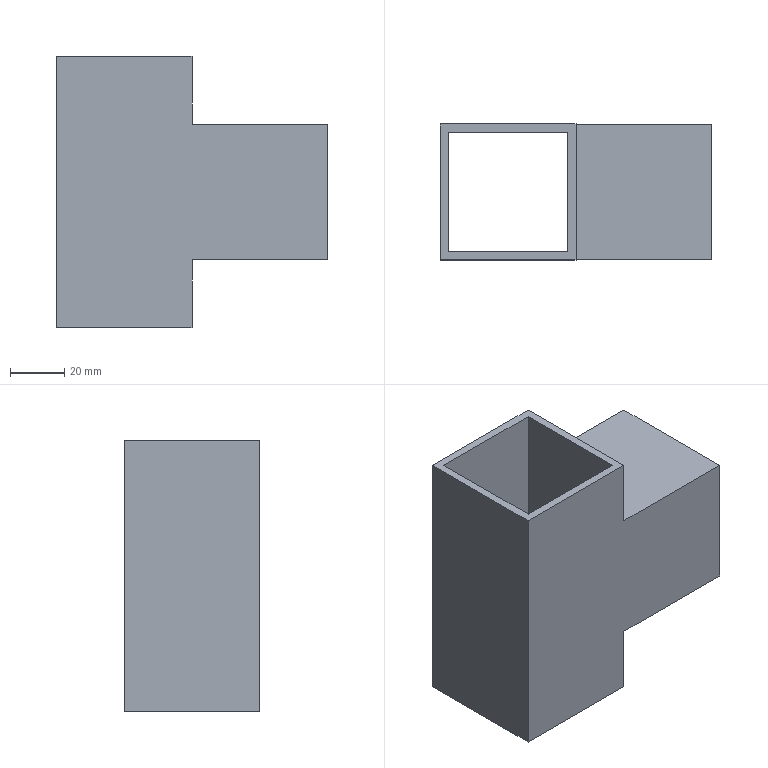Part | SolidWorks | features ICE 3, Extrusion 1 | 1 solid | 19 faces | box 100 x 50 x 100 mm | volume 84600 mm3 | plane 19
STEP:
#1=CARTESIAN_POINT('',(50.,0.,100.));
#2=VERTEX_POINT('',#1);
#3=CARTESIAN_POINT('',(50.,0.,75.));
#4=VERTEX_POINT('',#3);
#5=CARTESIAN_POINT('',(50.,0.,200.));
#6=DIRECTION('',(0.,0.,-1.));
#7=VECTOR('',#6,1000.);
#8=LINE('',#5,#7);
#9=EDGE_CURVE('',#2,#4,#8,.T.);
#10=ORIENTED_EDGE('',*,*,#9,.T.);
#11=CARTESIAN_POINT('',(50.,50.,75.));
#12=VERTEX_POINT('',#11);
#13=CARTESIAN_POINT('',(50.,50.,75.));
#14=DIRECTION('',(0.,1.,0.));
#15=VECTOR('',#14,1000.);
#16=LINE('',#13,#15);
#17=EDGE_CURVE('',#4,#12,#16,.T.);
#18=ORIENTED_EDGE('',*,*,#17,.T.);
#19=CARTESIAN_POINT('',(50.,50.,100.));
#20=VERTEX_POINT('',#19);
#21=CARTESIAN_POINT('',(50.,50.,200.));
#22=DIRECTION('',(0.,0.,-1.));
#23=VECTOR('',#22,1000.);
#24=LINE('',#21,#23);
#25=EDGE_CURVE('',#20,#12,#24,.T.);
#26=ORIENTED_EDGE('',*,*,#25,.F.);
#27=CARTESIAN_POINT('',(50.,50.,100.));
#28=DIRECTION('',(0.,1.,0.));
#29=VECTOR('',#28,1000.);
#30=LINE('',#27,#29);
#31=EDGE_CURVE('',#2,#20,#30,.T.);
#32=ORIENTED_EDGE('',*,*,#31,.F.);
#33=EDGE_LOOP('',(#10,#18,#26,#32));
#34=FACE_OUTER_BOUND('',#33,.T.);
#35=CARTESIAN_POINT('',(50.,50.,200.));
#36=DIRECTION('',(-1.,0.,0.));
#37=DIRECTION('',(0.,0.,1.));
#38=AXIS2_PLACEMENT_3D('',#35,#36,#37);
#39=PLANE('',#38);
#40=ADVANCED_FACE('',(#34),#39,.F.);
#41=CARTESIAN_POINT('',(50.,0.,25.));
#42=VERTEX_POINT('',#41);
#43=CARTESIAN_POINT('',(50.,0.,0.));
#44=VERTEX_POINT('',#43);
#45=CARTESIAN_POINT('',(50.,0.,200.));
#46=DIRECTION('',(0.,0.,-1.));
#47=VECTOR('',#46,1000.);
#48=LINE('',#45,#47);
#49=EDGE_CURVE('',#42,#44,#48,.T.);
#50=ORIENTED_EDGE('',*,*,#49,.F.);
#51=CARTESIAN_POINT('',(100.,0.,25.));
#52=VERTEX_POINT('',#51);
#53=CARTESIAN_POINT('',(100.,0.,25.));
#54=DIRECTION('',(-1.,0.,0.));
#55=VECTOR('',#54,1000.);
#56=LINE('',#53,#55);
#57=EDGE_CURVE('',#52,#42,#56,.T.);
#58=ORIENTED_EDGE('',*,*,#57,.F.);
#59=CARTESIAN_POINT('',(100.,0.,75.));
#60=VERTEX_POINT('',#59);
#61=CARTESIAN_POINT('',(100.,0.,75.));
#62=DIRECTION('',(0.,0.,1.));
#63=VECTOR('',#62,1000.);
#64=LINE('',#61,#63);
#65=EDGE_CURVE('',#52,#60,#64,.T.);
#66=ORIENTED_EDGE('',*,*,#65,.T.);
#67=CARTESIAN_POINT('',(100.,0.,75.));
#68=DIRECTION('',(-1.,0.,0.));
#69=VECTOR('',#68,1000.);
#70=LINE('',#67,#69);
#71=EDGE_CURVE('',#60,#4,#70,.T.);
#72=ORIENTED_EDGE('',*,*,#71,.T.);
#73=ORIENTED_EDGE('',*,*,#9,.F.);
#74=CARTESIAN_POINT('',(0.,0.,100.));
#75=VERTEX_POINT('',#74);
#76=CARTESIAN_POINT('',(50.,0.,100.));
#77=DIRECTION('',(1.,0.,0.));
#78=VECTOR('',#77,1000.);
#79=LINE('',#76,#78);
#80=EDGE_CURVE('',#75,#2,#79,.T.);
#81=ORIENTED_EDGE('',*,*,#80,.F.);
#82=CARTESIAN_POINT('',(0.,0.,0.));
#83=VERTEX_POINT('',#82);
#84=CARTESIAN_POINT('',(0.,0.,200.));
#85=DIRECTION('',(0.,0.,-1.));
#86=VECTOR('',#85,1000.);
#87=LINE('',#84,#86);
#88=EDGE_CURVE('',#75,#83,#87,.T.);
#89=ORIENTED_EDGE('',*,*,#88,.T.);
#90=CARTESIAN_POINT('',(50.,0.,0.));
#91=DIRECTION('',(1.,0.,0.));
#92=VECTOR('',#91,1000.);
#93=LINE('',#90,#92);
#94=EDGE_CURVE('',#83,#44,#93,.T.);
#95=ORIENTED_EDGE('',*,*,#94,.T.);
#96=EDGE_LOOP('',(#50,#58,#66,#72,#73,#81,#89,#95));
#97=FACE_OUTER_BOUND('',#96,.T.);
#98=CARTESIAN_POINT('',(50.,0.,200.));
#99=DIRECTION('',(0.,1.,0.));
#100=DIRECTION('',(0.,0.,1.));
#101=AXIS2_PLACEMENT_3D('',#98,#99,#100);
#102=PLANE('',#101);
#103=ADVANCED_FACE('',(#97),#102,.F.);
#104=CARTESIAN_POINT('',(50.,50.,25.));
#105=VERTEX_POINT('',#104);
#106=CARTESIAN_POINT('',(50.,50.,0.));
#107=VERTEX_POINT('',#106);
#108=CARTESIAN_POINT('',(50.,50.,200.));
#109=DIRECTION('',(0.,0.,-1.));
#110=VECTOR('',#109,1000.);
#111=LINE('',#108,#110);
#112=EDGE_CURVE('',#105,#107,#111,.T.);
#113=ORIENTED_EDGE('',*,*,#112,.F.);
#114=CARTESIAN_POINT('',(50.,50.,25.));
#115=DIRECTION('',(0.,-1.,0.));
#116=VECTOR('',#115,1000.);
#117=LINE('',#114,#116);
#118=EDGE_CURVE('',#105,#42,#117,.T.);
#119=ORIENTED_EDGE('',*,*,#118,.T.);
#120=ORIENTED_EDGE('',*,*,#49,.T.);
#121=CARTESIAN_POINT('',(50.,50.,0.));
#122=DIRECTION('',(0.,1.,0.));
#123=VECTOR('',#122,1000.);
#124=LINE('',#121,#123);
#125=EDGE_CURVE('',#44,#107,#124,.T.);
#126=ORIENTED_EDGE('',*,*,#125,.T.);
#127=EDGE_LOOP('',(#113,#119,#120,#126));
#128=FACE_OUTER_BOUND('',#127,.T.);
#129=CARTESIAN_POINT('',(50.,50.,200.));
#130=DIRECTION('',(-1.,0.,0.));
#131=DIRECTION('',(0.,0.,1.));
#132=AXIS2_PLACEMENT_3D('',#129,#130,#131);
#133=PLANE('',#132);
#134=ADVANCED_FACE('',(#128),#133,.F.);
#135=CARTESIAN_POINT('',(0.,50.,0.));
#136=VERTEX_POINT('',#135);
#137=CARTESIAN_POINT('',(0.,50.,0.));
#138=DIRECTION('',(-1.,0.,0.));
#139=VECTOR('',#138,1000.);
#140=LINE('',#137,#139);
#141=EDGE_CURVE('',#107,#136,#140,.T.);
#142=ORIENTED_EDGE('',*,*,#141,.T.);
#143=CARTESIAN_POINT('',(0.,50.,100.));
#144=VERTEX_POINT('',#143);
#145=CARTESIAN_POINT('',(0.,50.,200.));
#146=DIRECTION('',(0.,0.,-1.));
#147=VECTOR('',#146,1000.);
#148=LINE('',#145,#147);
#149=EDGE_CURVE('',#144,#136,#148,.T.);
#150=ORIENTED_EDGE('',*,*,#149,.F.);
#151=CARTESIAN_POINT('',(0.,50.,100.));
#152=DIRECTION('',(-1.,0.,0.));
#153=VECTOR('',#152,1000.);
#154=LINE('',#151,#153);
#155=EDGE_CURVE('',#20,#144,#154,.T.);
#156=ORIENTED_EDGE('',*,*,#155,.F.);
#157=ORIENTED_EDGE('',*,*,#25,.T.);
#158=CARTESIAN_POINT('',(100.,50.,75.));
#159=VERTEX_POINT('',#158);
#160=CARTESIAN_POINT('',(100.,50.,75.));
#161=DIRECTION('',(-1.,0.,0.));
#162=VECTOR('',#161,1000.);
#163=LINE('',#160,#162);
#164=EDGE_CURVE('',#159,#12,#163,.T.);
#165=ORIENTED_EDGE('',*,*,#164,.F.);
#166=CARTESIAN_POINT('',(100.,50.,25.));
#167=VERTEX_POINT('',#166);
#168=CARTESIAN_POINT('',(100.,50.,50.));
#169=DIRECTION('',(0.,0.,-1.));
#170=VECTOR('',#169,1000.);
#171=LINE('',#168,#170);
#172=EDGE_CURVE('',#159,#167,#171,.T.);
#173=ORIENTED_EDGE('',*,*,#172,.T.);
#174=CARTESIAN_POINT('',(100.,50.,25.));
#175=DIRECTION('',(-1.,0.,0.));
#176=VECTOR('',#175,1000.);
#177=LINE('',#174,#176);
#178=EDGE_CURVE('',#167,#105,#177,.T.);
#179=ORIENTED_EDGE('',*,*,#178,.T.);
#180=ORIENTED_EDGE('',*,*,#112,.T.);
#181=EDGE_LOOP('',(#142,#150,#156,#157,#165,#173,#179,#180));
#182=FACE_OUTER_BOUND('',#181,.T.);
#183=CARTESIAN_POINT('',(0.,50.,200.));
#184=DIRECTION('',(0.,-1.,0.));
#185=DIRECTION('',(0.,0.,-1.));
#186=AXIS2_PLACEMENT_3D('',#183,#184,#185);
#187=PLANE('',#186);
#188=ADVANCED_FACE('',(#182),#187,.F.);
#189=CARTESIAN_POINT('',(0.,0.,0.));
#190=DIRECTION('',(0.,-1.,0.));
#191=VECTOR('',#190,1000.);
#192=LINE('',#189,#191);
#193=EDGE_CURVE('',#136,#83,#192,.T.);
#194=ORIENTED_EDGE('',*,*,#193,.T.);
#195=ORIENTED_EDGE('',*,*,#88,.F.);
#196=CARTESIAN_POINT('',(0.,0.,100.));
#197=DIRECTION('',(0.,-1.,0.));
#198=VECTOR('',#197,1000.);
#199=LINE('',#196,#198);
#200=EDGE_CURVE('',#144,#75,#199,.T.);
#201=ORIENTED_EDGE('',*,*,#200,.F.);
#202=ORIENTED_EDGE('',*,*,#149,.T.);
#203=EDGE_LOOP('',(#194,#195,#201,#202));
#204=FACE_OUTER_BOUND('',#203,.T.);
#205=CARTESIAN_POINT('',(0.,0.,200.));
#206=DIRECTION('',(1.,0.,0.));
#207=DIRECTION('',(0.,0.,-1.));
#208=AXIS2_PLACEMENT_3D('',#205,#206,#207);
#209=PLANE('',#208);
#210=ADVANCED_FACE('',(#204),#209,.F.);
#211=CARTESIAN_POINT('',(3.,3.,0.));
#212=VERTEX_POINT('',#211);
#213=CARTESIAN_POINT('',(47.,3.,0.));
#214=VERTEX_POINT('',#213);
#215=CARTESIAN_POINT('',(47.,3.,0.));
#216=DIRECTION('',(1.,0.,0.));
#217=VECTOR('',#216,1000.);
#218=LINE('',#215,#217);
#219=EDGE_CURVE('',#212,#214,#218,.T.);
#220=ORIENTED_EDGE('',*,*,#219,.F.);
#221=CARTESIAN_POINT('',(3.,3.,100.));
#222=VERTEX_POINT('',#221);
#223=CARTESIAN_POINT('',(3.,3.,200.));
#224=DIRECTION('',(0.,0.,-1.));
#225=VECTOR('',#224,1000.);
#226=LINE('',#223,#225);
#227=EDGE_CURVE('',#222,#212,#226,.T.);
#228=ORIENTED_EDGE('',*,*,#227,.F.);
#229=CARTESIAN_POINT('',(47.,3.,100.));
#230=VERTEX_POINT('',#229);
#231=CARTESIAN_POINT('',(47.,3.,100.));
#232=DIRECTION('',(1.,0.,0.));
#233=VECTOR('',#232,1000.);
#234=LINE('',#231,#233);
#235=EDGE_CURVE('',#222,#230,#234,.T.);
#236=ORIENTED_EDGE('',*,*,#235,.T.);
#237=CARTESIAN_POINT('',(47.,3.,200.));
#238=DIRECTION('',(0.,0.,-1.));
#239=VECTOR('',#238,1000.);
#240=LINE('',#237,#239);
#241=EDGE_CURVE('',#230,#214,#240,.T.);
#242=ORIENTED_EDGE('',*,*,#241,.T.);
#243=EDGE_LOOP('',(#220,#228,#236,#242));
#244=FACE_OUTER_BOUND('',#243,.T.);
#245=CARTESIAN_POINT('',(47.,3.,200.));
#246=DIRECTION('',(0.,1.,0.));
#247=DIRECTION('',(0.,0.,1.));
#248=AXIS2_PLACEMENT_3D('',#245,#246,#247);
#249=PLANE('',#248);
#250=ADVANCED_FACE('',(#244),#249,.T.);
#251=CARTESIAN_POINT('',(47.,47.,0.));
#252=VERTEX_POINT('',#251);
#253=CARTESIAN_POINT('',(47.,47.,0.));
#254=DIRECTION('',(0.,1.,0.));
#255=VECTOR('',#254,1000.);
#256=LINE('',#253,#255);
#257=EDGE_CURVE('',#214,#252,#256,.T.);
#258=ORIENTED_EDGE('',*,*,#257,.F.);
#259=ORIENTED_EDGE('',*,*,#241,.F.);
#260=CARTESIAN_POINT('',(47.,47.,100.));
#261=VERTEX_POINT('',#260);
#262=CARTESIAN_POINT('',(47.,47.,100.));
#263=DIRECTION('',(0.,1.,0.));
#264=VECTOR('',#263,1000.);
#265=LINE('',#262,#264);
#266=EDGE_CURVE('',#230,#261,#265,.T.);
#267=ORIENTED_EDGE('',*,*,#266,.T.);
#268=CARTESIAN_POINT('',(47.,47.,200.));
#269=DIRECTION('',(0.,0.,-1.));
#270=VECTOR('',#269,1000.);
#271=LINE('',#268,#270);
#272=EDGE_CURVE('',#261,#252,#271,.T.);
#273=ORIENTED_EDGE('',*,*,#272,.T.);
#274=EDGE_LOOP('',(#258,#259,#267,#273));
#275=FACE_OUTER_BOUND('',#274,.T.);
#276=CARTESIAN_POINT('',(47.,47.,200.));
#277=DIRECTION('',(-1.,0.,0.));
#278=DIRECTION('',(0.,0.,1.));
#279=AXIS2_PLACEMENT_3D('',#276,#277,#278);
#280=PLANE('',#279);
#281=ADVANCED_FACE('',(#275),#280,.T.);
#282=CARTESIAN_POINT('',(3.,47.,0.));
#283=VERTEX_POINT('',#282);
#284=CARTESIAN_POINT('',(3.,47.,0.));
#285=DIRECTION('',(-1.,0.,0.));
#286=VECTOR('',#285,1000.);
#287=LINE('',#284,#286);
#288=EDGE_CURVE('',#252,#283,#287,.T.);
#289=ORIENTED_EDGE('',*,*,#288,.F.);
#290=ORIENTED_EDGE('',*,*,#272,.F.);
#291=CARTESIAN_POINT('',(3.,47.,100.));
#292=VERTEX_POINT('',#291);
#293=CARTESIAN_POINT('',(3.,47.,100.));
#294=DIRECTION('',(-1.,0.,0.));
#295=VECTOR('',#294,1000.);
#296=LINE('',#293,#295);
#297=EDGE_CURVE('',#261,#292,#296,.T.);
#298=ORIENTED_EDGE('',*,*,#297,.T.);
#299=CARTESIAN_POINT('',(3.,47.,200.));
#300=DIRECTION('',(0.,0.,-1.));
#301=VECTOR('',#300,1000.);
#302=LINE('',#299,#301);
#303=EDGE_CURVE('',#292,#283,#302,.T.);
#304=ORIENTED_EDGE('',*,*,#303,.T.);
#305=EDGE_LOOP('',(#289,#290,#298,#304));
#306=FACE_OUTER_BOUND('',#305,.T.);
#307=CARTESIAN_POINT('',(3.,47.,200.));
#308=DIRECTION('',(0.,-1.,0.));
#309=DIRECTION('',(0.,0.,-1.));
#310=AXIS2_PLACEMENT_3D('',#307,#308,#309);
#311=PLANE('',#310);
#312=ADVANCED_FACE('',(#306),#311,.T.);
#313=CARTESIAN_POINT('',(3.,3.,0.));
#314=DIRECTION('',(0.,-1.,0.));
#315=VECTOR('',#314,1000.);
#316=LINE('',#313,#315);
#317=EDGE_CURVE('',#283,#212,#316,.T.);
#318=ORIENTED_EDGE('',*,*,#317,.F.);
#319=ORIENTED_EDGE('',*,*,#303,.F.);
#320=CARTESIAN_POINT('',(3.,3.,100.));
#321=DIRECTION('',(0.,-1.,0.));
#322=VECTOR('',#321,1000.);
#323=LINE('',#320,#322);
#324=EDGE_CURVE('',#292,#222,#323,.T.);
#325=ORIENTED_EDGE('',*,*,#324,.T.);
#326=ORIENTED_EDGE('',*,*,#227,.T.);
#327=EDGE_LOOP('',(#318,#319,#325,#326));
#328=FACE_OUTER_BOUND('',#327,.T.);
#329=CARTESIAN_POINT('',(3.,3.,200.));
#330=DIRECTION('',(1.,0.,0.));
#331=DIRECTION('',(0.,0.,-1.));
#332=AXIS2_PLACEMENT_3D('',#329,#330,#331);
#333=PLANE('',#332);
#334=ADVANCED_FACE('',(#328),#333,.T.);
#335=ORIENTED_EDGE('',*,*,#94,.F.);
#336=ORIENTED_EDGE('',*,*,#193,.F.);
#337=ORIENTED_EDGE('',*,*,#141,.F.);
#338=ORIENTED_EDGE('',*,*,#125,.F.);
#339=EDGE_LOOP('',(#335,#336,#337,#338));
#340=FACE_OUTER_BOUND('',#339,.T.);
#341=ORIENTED_EDGE('',*,*,#317,.T.);
#342=ORIENTED_EDGE('',*,*,#219,.T.);
#343=ORIENTED_EDGE('',*,*,#257,.T.);
#344=ORIENTED_EDGE('',*,*,#288,.T.);
#345=EDGE_LOOP('',(#341,#342,#343,#344));
#346=FACE_BOUND('',#345,.T.);
#347=CARTESIAN_POINT('',(0.,0.,0.));
#348=DIRECTION('',(0.,0.,-1.));
#349=DIRECTION('',(-1.,0.,0.));
#350=AXIS2_PLACEMENT_3D('',#347,#348,#349);
#351=PLANE('',#350);
#352=ADVANCED_FACE('',(#340,#346),#351,.T.);
#353=ORIENTED_EDGE('',*,*,#324,.F.);
#354=ORIENTED_EDGE('',*,*,#297,.F.);
#355=ORIENTED_EDGE('',*,*,#266,.F.);
#356=ORIENTED_EDGE('',*,*,#235,.F.);
#357=EDGE_LOOP('',(#353,#354,#355,#356));
#358=FACE_BOUND('',#357,.T.);
#359=ORIENTED_EDGE('',*,*,#80,.T.);
#360=ORIENTED_EDGE('',*,*,#31,.T.);
#361=ORIENTED_EDGE('',*,*,#155,.T.);
#362=ORIENTED_EDGE('',*,*,#200,.T.);
#363=EDGE_LOOP('',(#359,#360,#361,#362));
#364=FACE_OUTER_BOUND('',#363,.T.);
#365=CARTESIAN_POINT('',(0.,0.,100.));
#366=DIRECTION('',(0.,0.,1.));
#367=DIRECTION('',(1.,0.,0.));
#368=AXIS2_PLACEMENT_3D('',#365,#366,#367);
#369=PLANE('',#368);
#370=ADVANCED_FACE('',(#358,#364),#369,.T.);
#371=ORIENTED_EDGE('',*,*,#17,.F.);
#372=ORIENTED_EDGE('',*,*,#71,.F.);
#373=CARTESIAN_POINT('',(100.,50.,75.));
#374=DIRECTION('',(0.,1.,0.));
#375=VECTOR('',#374,1000.);
#376=LINE('',#373,#375);
#377=EDGE_CURVE('',#60,#159,#376,.T.);
#378=ORIENTED_EDGE('',*,*,#377,.T.);
#379=ORIENTED_EDGE('',*,*,#164,.T.);
#380=EDGE_LOOP('',(#371,#372,#378,#379));
#381=FACE_OUTER_BOUND('',#380,.T.);
#382=CARTESIAN_POINT('',(100.,50.,75.));
#383=DIRECTION('',(0.,0.,1.));
#384=DIRECTION('',(1.,0.,0.));
#385=AXIS2_PLACEMENT_3D('',#382,#383,#384);
#386=PLANE('',#385);
#387=ADVANCED_FACE('',(#381),#386,.T.);
#388=ORIENTED_EDGE('',*,*,#118,.F.);
#389=ORIENTED_EDGE('',*,*,#178,.F.);
#390=CARTESIAN_POINT('',(100.,0.,25.));
#391=DIRECTION('',(0.,-1.,0.));
#392=VECTOR('',#391,1000.);
#393=LINE('',#390,#392);
#394=EDGE_CURVE('',#167,#52,#393,.T.);
#395=ORIENTED_EDGE('',*,*,#394,.T.);
#396=ORIENTED_EDGE('',*,*,#57,.T.);
#397=EDGE_LOOP('',(#388,#389,#395,#396));
#398=FACE_OUTER_BOUND('',#397,.T.);
#399=CARTESIAN_POINT('',(100.,0.,25.));
#400=DIRECTION('',(0.,0.,-1.));
#401=DIRECTION('',(0.,1.,0.));
#402=AXIS2_PLACEMENT_3D('',#399,#400,#401);
#403=PLANE('',#402);
#404=ADVANCED_FACE('',(#398),#403,.T.);
#405=CARTESIAN_POINT('',(100.,3.,72.));
#406=VERTEX_POINT('',#405);
#407=CARTESIAN_POINT('',(50.,3.,72.));
#408=VERTEX_POINT('',#407);
#409=CARTESIAN_POINT('',(100.,3.,72.));
#410=DIRECTION('',(-1.,0.,0.));
#411=VECTOR('',#410,1000.);
#412=LINE('',#409,#411);
#413=EDGE_CURVE('',#406,#408,#412,.T.);
#414=ORIENTED_EDGE('',*,*,#413,.T.);
#415=CARTESIAN_POINT('',(50.,47.,72.));
#416=VERTEX_POINT('',#415);
#417=CARTESIAN_POINT('',(50.,50.,72.));
#418=DIRECTION('',(0.,1.,0.));
#419=VECTOR('',#418,1000.);
#420=LINE('',#417,#419);
#421=EDGE_CURVE('',#408,#416,#420,.T.);
#422=ORIENTED_EDGE('',*,*,#421,.T.);
#423=CARTESIAN_POINT('',(100.,47.,72.));
#424=VERTEX_POINT('',#423);
#425=CARTESIAN_POINT('',(100.,47.,72.));
#426=DIRECTION('',(-1.,0.,0.));
#427=VECTOR('',#426,1000.);
#428=LINE('',#425,#427);
#429=EDGE_CURVE('',#424,#416,#428,.T.);
#430=ORIENTED_EDGE('',*,*,#429,.F.);
#431=CARTESIAN_POINT('',(100.,47.,72.));
#432=DIRECTION('',(0.,1.,0.));
#433=VECTOR('',#432,1000.);
#434=LINE('',#431,#433);
#435=EDGE_CURVE('',#406,#424,#434,.T.);
#436=ORIENTED_EDGE('',*,*,#435,.F.);
#437=EDGE_LOOP('',(#414,#422,#430,#436));
#438=FACE_OUTER_BOUND('',#437,.T.);
#439=CARTESIAN_POINT('',(100.,47.,72.));
#440=DIRECTION('',(0.,0.,1.));
#441=DIRECTION('',(1.,0.,0.));
#442=AXIS2_PLACEMENT_3D('',#439,#440,#441);
#443=PLANE('',#442);
#444=ADVANCED_FACE('',(#438),#443,.F.);
#445=CARTESIAN_POINT('',(100.,3.,28.));
#446=VERTEX_POINT('',#445);
#447=CARTESIAN_POINT('',(50.,3.,28.));
#448=VERTEX_POINT('',#447);
#449=CARTESIAN_POINT('',(100.,3.,28.));
#450=DIRECTION('',(-1.,0.,0.));
#451=VECTOR('',#450,1000.);
#452=LINE('',#449,#451);
#453=EDGE_CURVE('',#446,#448,#452,.T.);
#454=ORIENTED_EDGE('',*,*,#453,.T.);
#455=CARTESIAN_POINT('',(50.,3.,200.));
#456=DIRECTION('',(0.,0.,1.));
#457=VECTOR('',#456,1000.);
#458=LINE('',#455,#457);
#459=EDGE_CURVE('',#448,#408,#458,.T.);
#460=ORIENTED_EDGE('',*,*,#459,.T.);
#461=ORIENTED_EDGE('',*,*,#413,.F.);
#462=CARTESIAN_POINT('',(100.,3.,72.));
#463=DIRECTION('',(0.,0.,1.));
#464=VECTOR('',#463,1000.);
#465=LINE('',#462,#464);
#466=EDGE_CURVE('',#446,#406,#465,.T.);
#467=ORIENTED_EDGE('',*,*,#466,.F.);
#468=EDGE_LOOP('',(#454,#460,#461,#467));
#469=FACE_OUTER_BOUND('',#468,.T.);
#470=CARTESIAN_POINT('',(100.,3.,72.));
#471=DIRECTION('',(0.,-1.,0.));
#472=DIRECTION('',(0.,0.,-1.));
#473=AXIS2_PLACEMENT_3D('',#470,#471,#472);
#474=PLANE('',#473);
#475=ADVANCED_FACE('',(#469),#474,.F.);
#476=CARTESIAN_POINT('',(100.,47.,28.));
#477=VERTEX_POINT('',#476);
#478=CARTESIAN_POINT('',(50.,47.,28.));
#479=VERTEX_POINT('',#478);
#480=CARTESIAN_POINT('',(100.,47.,28.));
#481=DIRECTION('',(-1.,0.,0.));
#482=VECTOR('',#481,1000.);
#483=LINE('',#480,#482);
#484=EDGE_CURVE('',#477,#479,#483,.T.);
#485=ORIENTED_EDGE('',*,*,#484,.T.);
#486=CARTESIAN_POINT('',(50.,50.,28.));
#487=DIRECTION('',(0.,-1.,0.));
#488=VECTOR('',#487,1000.);
#489=LINE('',#486,#488);
#490=EDGE_CURVE('',#479,#448,#489,.T.);
#491=ORIENTED_EDGE('',*,*,#490,.T.);
#492=ORIENTED_EDGE('',*,*,#453,.F.);
#493=CARTESIAN_POINT('',(100.,3.,28.));
#494=DIRECTION('',(0.,-1.,0.));
#495=VECTOR('',#494,1000.);
#496=LINE('',#493,#495);
#497=EDGE_CURVE('',#477,#446,#496,.T.);
#498=ORIENTED_EDGE('',*,*,#497,.F.);
#499=EDGE_LOOP('',(#485,#491,#492,#498));
#500=FACE_OUTER_BOUND('',#499,.T.);
#501=CARTESIAN_POINT('',(100.,3.,28.));
#502=DIRECTION('',(0.,0.,-1.));
#503=DIRECTION('',(-1.,0.,0.));
#504=AXIS2_PLACEMENT_3D('',#501,#502,#503);
#505=PLANE('',#504);
#506=ADVANCED_FACE('',(#500),#505,.F.);
#507=ORIENTED_EDGE('',*,*,#429,.T.);
#508=CARTESIAN_POINT('',(50.,47.,200.));
#509=DIRECTION('',(0.,0.,-1.));
#510=VECTOR('',#509,1000.);
#511=LINE('',#508,#510);
#512=EDGE_CURVE('',#416,#479,#511,.T.);
#513=ORIENTED_EDGE('',*,*,#512,.T.);
#514=ORIENTED_EDGE('',*,*,#484,.F.);
#515=CARTESIAN_POINT('',(100.,47.,50.));
#516=DIRECTION('',(0.,0.,-1.));
#517=VECTOR('',#516,1000.);
#518=LINE('',#515,#517);
#519=EDGE_CURVE('',#424,#477,#518,.T.);
#520=ORIENTED_EDGE('',*,*,#519,.F.);
#521=EDGE_LOOP('',(#507,#513,#514,#520));
#522=FACE_OUTER_BOUND('',#521,.T.);
#523=CARTESIAN_POINT('',(100.,47.,50.));
#524=DIRECTION('',(0.,1.,0.));
#525=DIRECTION('',(0.,0.,1.));
#526=AXIS2_PLACEMENT_3D('',#523,#524,#525);
#527=PLANE('',#526);
#528=ADVANCED_FACE('',(#522),#527,.F.);
#529=ORIENTED_EDGE('',*,*,#435,.T.);
#530=ORIENTED_EDGE('',*,*,#519,.T.);
#531=ORIENTED_EDGE('',*,*,#497,.T.);
#532=ORIENTED_EDGE('',*,*,#466,.T.);
#533=EDGE_LOOP('',(#529,#530,#531,#532));
#534=FACE_BOUND('',#533,.T.);
#535=ORIENTED_EDGE('',*,*,#172,.F.);
#536=ORIENTED_EDGE('',*,*,#377,.F.);
#537=ORIENTED_EDGE('',*,*,#65,.F.);
#538=ORIENTED_EDGE('',*,*,#394,.F.);
#539=EDGE_LOOP('',(#535,#536,#537,#538));
#540=FACE_OUTER_BOUND('',#539,.T.);
#541=CARTESIAN_POINT('',(100.,0.,0.));
#542=DIRECTION('',(1.,0.,0.));
#543=DIRECTION('',(0.,0.,-1.));
#544=AXIS2_PLACEMENT_3D('',#541,#542,#543);
#545=PLANE('',#544);
#546=ADVANCED_FACE('',(#534,#540),#545,.T.);
#547=ORIENTED_EDGE('',*,*,#421,.F.);
#548=ORIENTED_EDGE('',*,*,#459,.F.);
#549=ORIENTED_EDGE('',*,*,#490,.F.);
#550=ORIENTED_EDGE('',*,*,#512,.F.);
#551=EDGE_LOOP('',(#547,#548,#549,#550));
#552=FACE_OUTER_BOUND('',#551,.T.);
#553=CARTESIAN_POINT('',(50.,50.,200.));
#554=DIRECTION('',(-1.,0.,0.));
#555=DIRECTION('',(0.,0.,1.));
#556=AXIS2_PLACEMENT_3D('',#553,#554,#555);
#557=PLANE('',#556);
#558=ADVANCED_FACE('',(#552),#557,.F.);
#559=CLOSED_SHELL('',(#40,#103,#134,#188,#210,#250,#281,#312,#334,#352,#370,#387,#404,#444,#475,#506,#528,#546,#558));
#560=MANIFOLD_SOLID_BREP('',#559);
#561=CARTESIAN_POINT('',(0.,0.,0.));
#562=DIRECTION('',(0.,0.,1.));
#563=DIRECTION('',(1.,0.,0.));
#564=AXIS2_PLACEMENT_3D('',#561,#562,#563);
#565=(LENGTH_UNIT()NAMED_UNIT(*)SI_UNIT(.MILLI.,.METRE.));
#566=UNCERTAINTY_MEASURE_WITH_UNIT(LENGTH_MEASURE(0.00001),#565,'','');
#567=(NAMED_UNIT(*)PLANE_ANGLE_UNIT()SI_UNIT($,.RADIAN.));
#568=(NAMED_UNIT(*)SI_UNIT($,.STERADIAN.)SOLID_ANGLE_UNIT());
#569=(GEOMETRIC_REPRESENTATION_CONTEXT(3)GLOBAL_UNCERTAINTY_ASSIGNED_CONTEXT((#566))GLOBAL_UNIT_ASSIGNED_CONTEXT((#565,#567,#568))REPRESENTATION_CONTEXT('',''));
#570=ADVANCED_BREP_SHAPE_REPRESENTATION('',(#560,#564),#569);